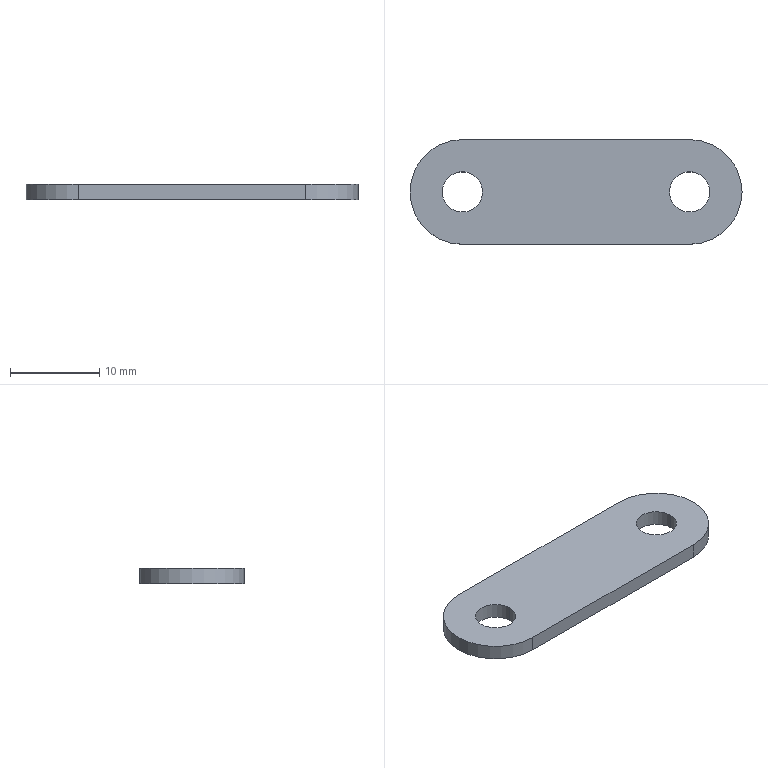Part | STEP file | CHAIN-02_1_02LT_1-2 | 1 solid | 11 faces | box 37.1 x 11.7 x 1.7 mm | volume 633.904 mm3 | cylinder 7 | plane 4 | commonest cylinder face diameters 4.5 x4 11.7 x3
STEP:
#1=CARTESIAN_POINT('',(-14.95,0.,0.));
#2=VERTEX_POINT('',#1);
#3=CARTESIAN_POINT('',(-10.45,0.,0.));
#4=VERTEX_POINT('',#3);
#5=CARTESIAN_POINT('',(-12.7,0.,0.));
#6=DIRECTION('',(0.,0.,1.));
#7=DIRECTION('',(1.,0.,0.));
#8=AXIS2_PLACEMENT_3D('',#5,#6,#7);
#9=CIRCLE('',#8,2.25);
#10=EDGE_CURVE('',#2,#4,#9,.T.);
#11=ORIENTED_EDGE('',*,*,#10,.F.);
#12=CARTESIAN_POINT('',(-14.95,0.,1.7));
#13=VERTEX_POINT('',#12);
#14=CARTESIAN_POINT('',(-14.95,0.,0.));
#15=DIRECTION('',(0.,0.,1.));
#16=VECTOR('',#15,1000.);
#17=LINE('',#14,#16);
#18=EDGE_CURVE('',#2,#13,#17,.T.);
#19=ORIENTED_EDGE('',*,*,#18,.T.);
#20=CARTESIAN_POINT('',(-10.45,0.,1.7));
#21=VERTEX_POINT('',#20);
#22=CARTESIAN_POINT('',(-12.7,0.,1.7));
#23=DIRECTION('',(0.,0.,-1.));
#24=DIRECTION('',(1.,0.,0.));
#25=AXIS2_PLACEMENT_3D('',#22,#23,#24);
#26=CIRCLE('',#25,2.25);
#27=EDGE_CURVE('',#21,#13,#26,.T.);
#28=ORIENTED_EDGE('',*,*,#27,.F.);
#29=CARTESIAN_POINT('',(-10.45,0.,0.));
#30=DIRECTION('',(0.,0.,1.));
#31=VECTOR('',#30,1000.);
#32=LINE('',#29,#31);
#33=EDGE_CURVE('',#4,#21,#32,.T.);
#34=ORIENTED_EDGE('',*,*,#33,.F.);
#35=EDGE_LOOP('',(#11,#19,#28,#34));
#36=FACE_OUTER_BOUND('',#35,.T.);
#37=CARTESIAN_POINT('',(-12.7,0.,0.));
#38=DIRECTION('',(0.,0.,1.));
#39=DIRECTION('',(1.,0.,0.));
#40=AXIS2_PLACEMENT_3D('',#37,#38,#39);
#41=CYLINDRICAL_SURFACE('',#40,2.25);
#42=ADVANCED_FACE('',(#36),#41,.F.);
#43=CARTESIAN_POINT('',(10.45,0.,0.));
#44=VERTEX_POINT('',#43);
#45=CARTESIAN_POINT('',(14.95,0.,0.));
#46=VERTEX_POINT('',#45);
#47=CARTESIAN_POINT('',(12.7,0.,0.));
#48=DIRECTION('',(0.,0.,1.));
#49=DIRECTION('',(1.,0.,0.));
#50=AXIS2_PLACEMENT_3D('',#47,#48,#49);
#51=CIRCLE('',#50,2.25);
#52=EDGE_CURVE('',#44,#46,#51,.T.);
#53=ORIENTED_EDGE('',*,*,#52,.F.);
#54=CARTESIAN_POINT('',(10.45,0.,1.7));
#55=VERTEX_POINT('',#54);
#56=CARTESIAN_POINT('',(10.45,0.,0.));
#57=DIRECTION('',(0.,0.,1.));
#58=VECTOR('',#57,1000.);
#59=LINE('',#56,#58);
#60=EDGE_CURVE('',#44,#55,#59,.T.);
#61=ORIENTED_EDGE('',*,*,#60,.T.);
#62=CARTESIAN_POINT('',(14.95,0.,1.7));
#63=VERTEX_POINT('',#62);
#64=CARTESIAN_POINT('',(12.7,0.,1.7));
#65=DIRECTION('',(0.,0.,-1.));
#66=DIRECTION('',(1.,0.,0.));
#67=AXIS2_PLACEMENT_3D('',#64,#65,#66);
#68=CIRCLE('',#67,2.25);
#69=EDGE_CURVE('',#63,#55,#68,.T.);
#70=ORIENTED_EDGE('',*,*,#69,.F.);
#71=CARTESIAN_POINT('',(14.95,0.,0.));
#72=DIRECTION('',(0.,0.,1.));
#73=VECTOR('',#72,1000.);
#74=LINE('',#71,#73);
#75=EDGE_CURVE('',#46,#63,#74,.T.);
#76=ORIENTED_EDGE('',*,*,#75,.F.);
#77=EDGE_LOOP('',(#53,#61,#70,#76));
#78=FACE_OUTER_BOUND('',#77,.T.);
#79=CARTESIAN_POINT('',(12.7,0.,0.));
#80=DIRECTION('',(0.,0.,1.));
#81=DIRECTION('',(1.,0.,0.));
#82=AXIS2_PLACEMENT_3D('',#79,#80,#81);
#83=CYLINDRICAL_SURFACE('',#82,2.25);
#84=ADVANCED_FACE('',(#78),#83,.F.);
#85=CARTESIAN_POINT('',(12.7,-5.85,0.));
#86=VERTEX_POINT('',#85);
#87=CARTESIAN_POINT('',(18.55,0.,0.));
#88=VERTEX_POINT('',#87);
#89=CARTESIAN_POINT('',(12.7,0.,0.));
#90=DIRECTION('',(0.,0.,1.));
#91=DIRECTION('',(1.,0.,0.));
#92=AXIS2_PLACEMENT_3D('',#89,#90,#91);
#93=CIRCLE('',#92,5.85);
#94=EDGE_CURVE('',#86,#88,#93,.T.);
#95=ORIENTED_EDGE('',*,*,#94,.T.);
#96=CARTESIAN_POINT('',(18.55,0.,1.7));
#97=VERTEX_POINT('',#96);
#98=CARTESIAN_POINT('',(18.55,0.,0.));
#99=DIRECTION('',(0.,0.,1.));
#100=VECTOR('',#99,1000.);
#101=LINE('',#98,#100);
#102=EDGE_CURVE('',#88,#97,#101,.T.);
#103=ORIENTED_EDGE('',*,*,#102,.T.);
#104=CARTESIAN_POINT('',(12.7,-5.85,1.7));
#105=VERTEX_POINT('',#104);
#106=CARTESIAN_POINT('',(12.7,0.,1.7));
#107=DIRECTION('',(0.,0.,1.));
#108=DIRECTION('',(1.,0.,0.));
#109=AXIS2_PLACEMENT_3D('',#106,#107,#108);
#110=CIRCLE('',#109,5.85);
#111=EDGE_CURVE('',#105,#97,#110,.T.);
#112=ORIENTED_EDGE('',*,*,#111,.F.);
#113=CARTESIAN_POINT('',(12.7,-5.85,0.));
#114=DIRECTION('',(0.,0.,-1.));
#115=VECTOR('',#114,1000.);
#116=LINE('',#113,#115);
#117=EDGE_CURVE('',#105,#86,#116,.T.);
#118=ORIENTED_EDGE('',*,*,#117,.T.);
#119=EDGE_LOOP('',(#95,#103,#112,#118));
#120=FACE_OUTER_BOUND('',#119,.T.);
#121=CARTESIAN_POINT('',(12.7,0.,0.));
#122=DIRECTION('',(0.,0.,1.));
#123=DIRECTION('',(1.,0.,0.));
#124=AXIS2_PLACEMENT_3D('',#121,#122,#123);
#125=CYLINDRICAL_SURFACE('',#124,5.85);
#126=ADVANCED_FACE('',(#120),#125,.T.);
#127=ORIENTED_EDGE('',*,*,#27,.T.);
#128=CARTESIAN_POINT('',(-12.7,0.,1.7));
#129=DIRECTION('',(0.,0.,-1.));
#130=DIRECTION('',(1.,0.,0.));
#131=AXIS2_PLACEMENT_3D('',#128,#129,#130);
#132=CIRCLE('',#131,2.25);
#133=EDGE_CURVE('',#13,#21,#132,.T.);
#134=ORIENTED_EDGE('',*,*,#133,.T.);
#135=EDGE_LOOP('',(#127,#134));
#136=FACE_BOUND('',#135,.T.);
#137=ORIENTED_EDGE('',*,*,#69,.T.);
#138=CARTESIAN_POINT('',(12.7,0.,1.7));
#139=DIRECTION('',(0.,0.,-1.));
#140=DIRECTION('',(1.,0.,0.));
#141=AXIS2_PLACEMENT_3D('',#138,#139,#140);
#142=CIRCLE('',#141,2.25);
#143=EDGE_CURVE('',#55,#63,#142,.T.);
#144=ORIENTED_EDGE('',*,*,#143,.T.);
#145=EDGE_LOOP('',(#137,#144));
#146=FACE_BOUND('',#145,.T.);
#147=ORIENTED_EDGE('',*,*,#111,.T.);
#148=CARTESIAN_POINT('',(12.7,5.85,1.7));
#149=VERTEX_POINT('',#148);
#150=CARTESIAN_POINT('',(12.7,0.,1.7));
#151=DIRECTION('',(0.,0.,1.));
#152=DIRECTION('',(1.,0.,0.));
#153=AXIS2_PLACEMENT_3D('',#150,#151,#152);
#154=CIRCLE('',#153,5.85);
#155=EDGE_CURVE('',#97,#149,#154,.T.);
#156=ORIENTED_EDGE('',*,*,#155,.T.);
#157=CARTESIAN_POINT('',(-12.7,5.85,1.7));
#158=VERTEX_POINT('',#157);
#159=CARTESIAN_POINT('',(0.,5.85,1.7));
#160=DIRECTION('',(-1.,0.,0.));
#161=VECTOR('',#160,1000.);
#162=LINE('',#159,#161);
#163=EDGE_CURVE('',#149,#158,#162,.T.);
#164=ORIENTED_EDGE('',*,*,#163,.T.);
#165=CARTESIAN_POINT('',(-12.7,-5.85,1.7));
#166=VERTEX_POINT('',#165);
#167=CARTESIAN_POINT('',(-12.7,0.,1.7));
#168=DIRECTION('',(0.,0.,1.));
#169=DIRECTION('',(1.,0.,0.));
#170=AXIS2_PLACEMENT_3D('',#167,#168,#169);
#171=CIRCLE('',#170,5.85);
#172=EDGE_CURVE('',#158,#166,#171,.T.);
#173=ORIENTED_EDGE('',*,*,#172,.T.);
#174=CARTESIAN_POINT('',(0.,-5.85,1.7));
#175=DIRECTION('',(1.,0.,0.));
#176=VECTOR('',#175,1000.);
#177=LINE('',#174,#176);
#178=EDGE_CURVE('',#166,#105,#177,.T.);
#179=ORIENTED_EDGE('',*,*,#178,.T.);
#180=EDGE_LOOP('',(#147,#156,#164,#173,#179));
#181=FACE_OUTER_BOUND('',#180,.T.);
#182=CARTESIAN_POINT('',(0.,0.,1.7));
#183=DIRECTION('',(0.,0.,1.));
#184=DIRECTION('',(1.,0.,0.));
#185=AXIS2_PLACEMENT_3D('',#182,#183,#184);
#186=PLANE('',#185);
#187=ADVANCED_FACE('',(#136,#146,#181),#186,.T.);
#188=ORIENTED_EDGE('',*,*,#18,.F.);
#189=CARTESIAN_POINT('',(-12.7,0.,0.));
#190=DIRECTION('',(0.,0.,1.));
#191=DIRECTION('',(1.,0.,0.));
#192=AXIS2_PLACEMENT_3D('',#189,#190,#191);
#193=CIRCLE('',#192,2.25);
#194=EDGE_CURVE('',#4,#2,#193,.T.);
#195=ORIENTED_EDGE('',*,*,#194,.F.);
#196=ORIENTED_EDGE('',*,*,#33,.T.);
#197=ORIENTED_EDGE('',*,*,#133,.F.);
#198=EDGE_LOOP('',(#188,#195,#196,#197));
#199=FACE_OUTER_BOUND('',#198,.T.);
#200=CARTESIAN_POINT('',(-12.7,0.,0.));
#201=DIRECTION('',(0.,0.,1.));
#202=DIRECTION('',(1.,0.,0.));
#203=AXIS2_PLACEMENT_3D('',#200,#201,#202);
#204=CYLINDRICAL_SURFACE('',#203,2.25);
#205=ADVANCED_FACE('',(#199),#204,.F.);
#206=ORIENTED_EDGE('',*,*,#60,.F.);
#207=CARTESIAN_POINT('',(12.7,0.,0.));
#208=DIRECTION('',(0.,0.,1.));
#209=DIRECTION('',(1.,0.,0.));
#210=AXIS2_PLACEMENT_3D('',#207,#208,#209);
#211=CIRCLE('',#210,2.25);
#212=EDGE_CURVE('',#46,#44,#211,.T.);
#213=ORIENTED_EDGE('',*,*,#212,.F.);
#214=ORIENTED_EDGE('',*,*,#75,.T.);
#215=ORIENTED_EDGE('',*,*,#143,.F.);
#216=EDGE_LOOP('',(#206,#213,#214,#215));
#217=FACE_OUTER_BOUND('',#216,.T.);
#218=CARTESIAN_POINT('',(12.7,0.,0.));
#219=DIRECTION('',(0.,0.,1.));
#220=DIRECTION('',(1.,0.,0.));
#221=AXIS2_PLACEMENT_3D('',#218,#219,#220);
#222=CYLINDRICAL_SURFACE('',#221,2.25);
#223=ADVANCED_FACE('',(#217),#222,.F.);
#224=ORIENTED_EDGE('',*,*,#102,.F.);
#225=CARTESIAN_POINT('',(12.7,5.85,0.));
#226=VERTEX_POINT('',#225);
#227=CARTESIAN_POINT('',(12.7,0.,0.));
#228=DIRECTION('',(0.,0.,1.));
#229=DIRECTION('',(1.,0.,0.));
#230=AXIS2_PLACEMENT_3D('',#227,#228,#229);
#231=CIRCLE('',#230,5.85);
#232=EDGE_CURVE('',#88,#226,#231,.T.);
#233=ORIENTED_EDGE('',*,*,#232,.T.);
#234=CARTESIAN_POINT('',(12.7,5.85,0.));
#235=DIRECTION('',(0.,0.,1.));
#236=VECTOR('',#235,1000.);
#237=LINE('',#234,#236);
#238=EDGE_CURVE('',#226,#149,#237,.T.);
#239=ORIENTED_EDGE('',*,*,#238,.T.);
#240=ORIENTED_EDGE('',*,*,#155,.F.);
#241=EDGE_LOOP('',(#224,#233,#239,#240));
#242=FACE_OUTER_BOUND('',#241,.T.);
#243=CARTESIAN_POINT('',(12.7,0.,0.));
#244=DIRECTION('',(0.,0.,1.));
#245=DIRECTION('',(1.,0.,0.));
#246=AXIS2_PLACEMENT_3D('',#243,#244,#245);
#247=CYLINDRICAL_SURFACE('',#246,5.85);
#248=ADVANCED_FACE('',(#242),#247,.T.);
#249=ORIENTED_EDGE('',*,*,#117,.F.);
#250=ORIENTED_EDGE('',*,*,#178,.F.);
#251=CARTESIAN_POINT('',(-12.7,-5.85,0.));
#252=VERTEX_POINT('',#251);
#253=CARTESIAN_POINT('',(-12.7,-5.85,0.));
#254=DIRECTION('',(0.,0.,-1.));
#255=VECTOR('',#254,1000.);
#256=LINE('',#253,#255);
#257=EDGE_CURVE('',#166,#252,#256,.T.);
#258=ORIENTED_EDGE('',*,*,#257,.T.);
#259=CARTESIAN_POINT('',(-12.7,-5.85,0.));
#260=DIRECTION('',(1.,0.,0.));
#261=VECTOR('',#260,1000.);
#262=LINE('',#259,#261);
#263=EDGE_CURVE('',#252,#86,#262,.T.);
#264=ORIENTED_EDGE('',*,*,#263,.T.);
#265=EDGE_LOOP('',(#249,#250,#258,#264));
#266=FACE_OUTER_BOUND('',#265,.T.);
#267=CARTESIAN_POINT('',(-12.7,-5.85,0.));
#268=DIRECTION('',(0.,-1.,0.));
#269=DIRECTION('',(0.,0.,-1.));
#270=AXIS2_PLACEMENT_3D('',#267,#268,#269);
#271=PLANE('',#270);
#272=ADVANCED_FACE('',(#266),#271,.T.);
#273=ORIENTED_EDGE('',*,*,#257,.F.);
#274=ORIENTED_EDGE('',*,*,#172,.F.);
#275=CARTESIAN_POINT('',(-12.7,5.85,0.));
#276=VERTEX_POINT('',#275);
#277=CARTESIAN_POINT('',(-12.7,5.85,0.));
#278=DIRECTION('',(0.,0.,-1.));
#279=VECTOR('',#278,1000.);
#280=LINE('',#277,#279);
#281=EDGE_CURVE('',#158,#276,#280,.T.);
#282=ORIENTED_EDGE('',*,*,#281,.T.);
#283=CARTESIAN_POINT('',(-12.7,0.,0.));
#284=DIRECTION('',(0.,0.,1.));
#285=DIRECTION('',(1.,0.,0.));
#286=AXIS2_PLACEMENT_3D('',#283,#284,#285);
#287=CIRCLE('',#286,5.85);
#288=EDGE_CURVE('',#276,#252,#287,.T.);
#289=ORIENTED_EDGE('',*,*,#288,.T.);
#290=EDGE_LOOP('',(#273,#274,#282,#289));
#291=FACE_OUTER_BOUND('',#290,.T.);
#292=CARTESIAN_POINT('',(-12.7,0.,0.));
#293=DIRECTION('',(0.,0.,1.));
#294=DIRECTION('',(1.,0.,0.));
#295=AXIS2_PLACEMENT_3D('',#292,#293,#294);
#296=CYLINDRICAL_SURFACE('',#295,5.85);
#297=ADVANCED_FACE('',(#291),#296,.T.);
#298=ORIENTED_EDGE('',*,*,#281,.F.);
#299=ORIENTED_EDGE('',*,*,#163,.F.);
#300=ORIENTED_EDGE('',*,*,#238,.F.);
#301=CARTESIAN_POINT('',(12.7,5.85,0.));
#302=DIRECTION('',(-1.,0.,0.));
#303=VECTOR('',#302,1000.);
#304=LINE('',#301,#303);
#305=EDGE_CURVE('',#226,#276,#304,.T.);
#306=ORIENTED_EDGE('',*,*,#305,.T.);
#307=EDGE_LOOP('',(#298,#299,#300,#306));
#308=FACE_OUTER_BOUND('',#307,.T.);
#309=CARTESIAN_POINT('',(12.7,5.85,0.));
#310=DIRECTION('',(0.,1.,0.));
#311=DIRECTION('',(0.,0.,1.));
#312=AXIS2_PLACEMENT_3D('',#309,#310,#311);
#313=PLANE('',#312);
#314=ADVANCED_FACE('',(#308),#313,.T.);
#315=ORIENTED_EDGE('',*,*,#194,.T.);
#316=ORIENTED_EDGE('',*,*,#10,.T.);
#317=EDGE_LOOP('',(#315,#316));
#318=FACE_BOUND('',#317,.T.);
#319=ORIENTED_EDGE('',*,*,#212,.T.);
#320=ORIENTED_EDGE('',*,*,#52,.T.);
#321=EDGE_LOOP('',(#319,#320));
#322=FACE_BOUND('',#321,.T.);
#323=ORIENTED_EDGE('',*,*,#288,.F.);
#324=ORIENTED_EDGE('',*,*,#305,.F.);
#325=ORIENTED_EDGE('',*,*,#232,.F.);
#326=ORIENTED_EDGE('',*,*,#94,.F.);
#327=ORIENTED_EDGE('',*,*,#263,.F.);
#328=EDGE_LOOP('',(#323,#324,#325,#326,#327));
#329=FACE_OUTER_BOUND('',#328,.T.);
#330=CARTESIAN_POINT('',(0.,0.,0.));
#331=DIRECTION('',(0.,0.,1.));
#332=DIRECTION('',(1.,0.,0.));
#333=AXIS2_PLACEMENT_3D('',#330,#331,#332);
#334=PLANE('',#333);
#335=ADVANCED_FACE('',(#318,#322,#329),#334,.F.);
#336=CLOSED_SHELL('',(#42,#84,#126,#187,#205,#223,#248,#272,#297,#314,#335));
#337=MANIFOLD_SOLID_BREP('',#336);
#338=CARTESIAN_POINT('',(0.,0.,0.));
#339=DIRECTION('',(0.,0.,1.));
#340=DIRECTION('',(1.,0.,0.));
#341=AXIS2_PLACEMENT_3D('',#338,#339,#340);
#342=(LENGTH_UNIT()NAMED_UNIT(*)SI_UNIT(.MILLI.,.METRE.));
#343=UNCERTAINTY_MEASURE_WITH_UNIT(LENGTH_MEASURE(0.00001),#342,'','');
#344=(NAMED_UNIT(*)PLANE_ANGLE_UNIT()SI_UNIT($,.RADIAN.));
#345=(NAMED_UNIT(*)SI_UNIT($,.STERADIAN.)SOLID_ANGLE_UNIT());
#346=(GEOMETRIC_REPRESENTATION_CONTEXT(3)GLOBAL_UNCERTAINTY_ASSIGNED_CONTEXT((#343))GLOBAL_UNIT_ASSIGNED_CONTEXT((#342,#344,#345))REPRESENTATION_CONTEXT('',''));
#347=ADVANCED_BREP_SHAPE_REPRESENTATION('',(#337,#341),#346);